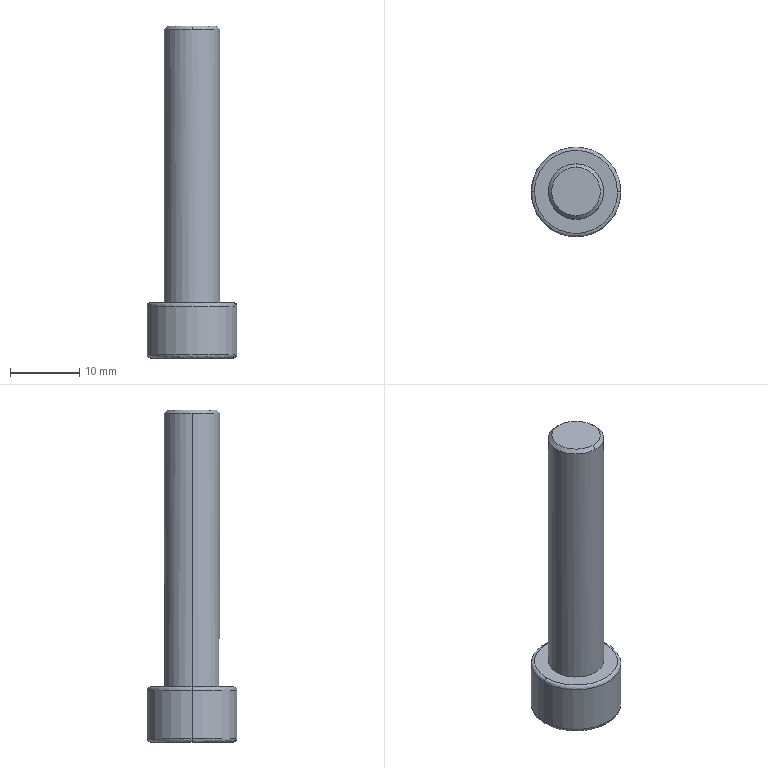Part | STEP file | Screw | 1 solid | 20 faces | box 13 x 13 x 48 mm | volume 2788 mm3 | plane 10 | spline 4 | cylinder 4 | cone 2 | commonest cylinder face diameters 8 x2 13 x2